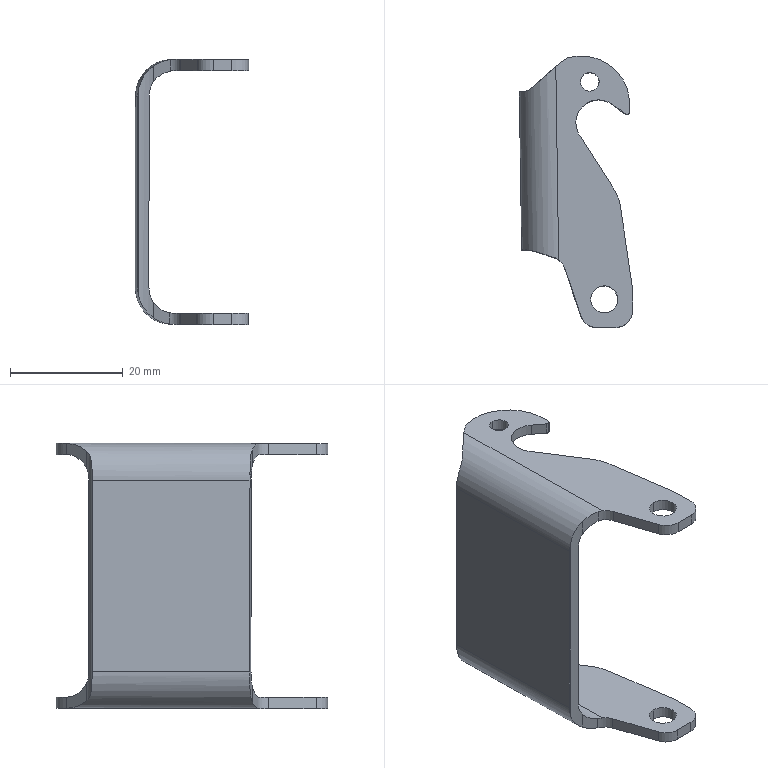Part | SolidWorks | features BaseBody 1 | 1 solid | 58 faces | box 20.1 x 48.212 x 47.031 mm | volume 4643 mm3 | cylinder 33 | plane 25 | commonest cylinder face diameters 6 x6 1 x4 3.3 x4 4.8 x4 16 x3 7.4 x2